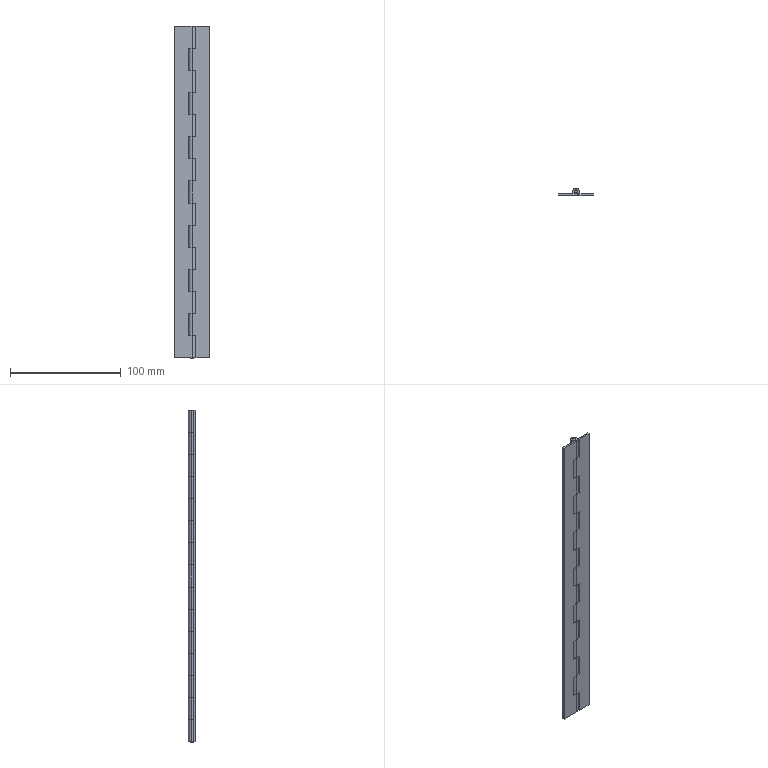Part | SolidWorks | features BaseBody 3 | 3 solids | 136 faces | box 32 x 6.5 x 300 mm | volume 21876 mm3 | cylinder 77 | plane 55 | cone 4 | commonest cylinder face diameters 6.5 x45 3.5 x32